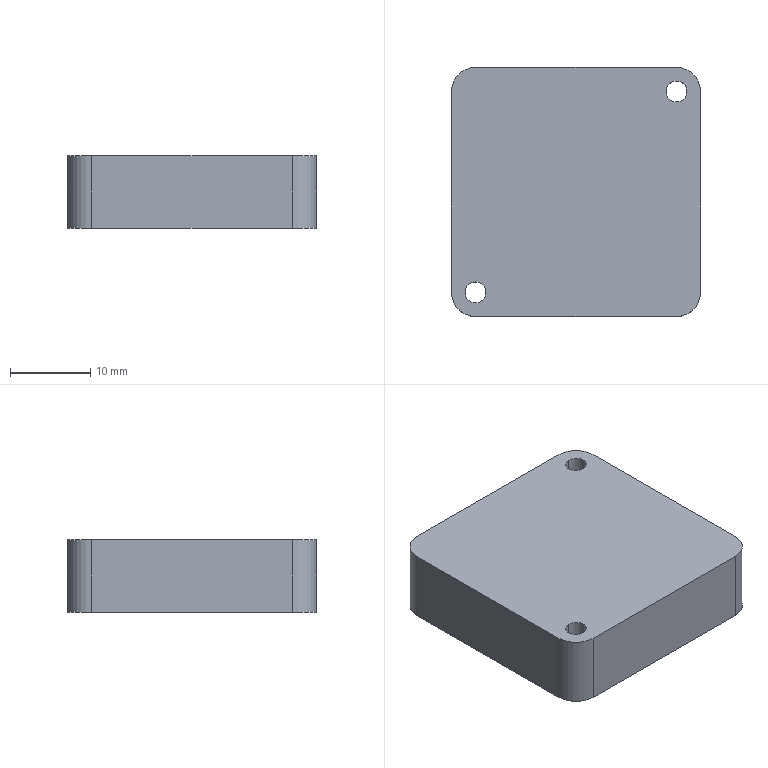Part | NX | 1 solid | 14 faces | box 31 x 31 x 9 mm | volume 8484 mm3 | cylinder 8 | plane 6 | commonest cylinder face diameters 2.6 x4 6 x4
STEP:
#1=CARTESIAN_POINT('',(15.5,12.5,0.));
#2=VERTEX_POINT('',#1);
#3=CARTESIAN_POINT('',(15.5,-12.5,0.));
#4=VERTEX_POINT('',#3);
#5=CARTESIAN_POINT('',(15.5,12.5,0.));
#6=DIRECTION('',(0.,-1.,0.));
#7=VECTOR('',#6,1000.);
#8=LINE('',#5,#7);
#9=EDGE_CURVE('',#2,#4,#8,.T.);
#10=ORIENTED_EDGE('',*,*,#9,.F.);
#11=CARTESIAN_POINT('',(12.5,15.5,0.));
#12=VERTEX_POINT('',#11);
#13=CARTESIAN_POINT('',(12.5,12.5,0.));
#14=DIRECTION('',(0.,0.,1.));
#15=DIRECTION('',(1.,0.,0.));
#16=AXIS2_PLACEMENT_3D('',#13,#14,#15);
#17=CIRCLE('',#16,3.);
#18=EDGE_CURVE('',#2,#12,#17,.T.);
#19=ORIENTED_EDGE('',*,*,#18,.T.);
#20=CARTESIAN_POINT('',(-12.5,15.5,0.));
#21=VERTEX_POINT('',#20);
#22=CARTESIAN_POINT('',(-12.5,15.5,0.));
#23=DIRECTION('',(1.,0.,0.));
#24=VECTOR('',#23,1000.);
#25=LINE('',#22,#24);
#26=EDGE_CURVE('',#21,#12,#25,.T.);
#27=ORIENTED_EDGE('',*,*,#26,.F.);
#28=CARTESIAN_POINT('',(-15.5,12.5,0.));
#29=VERTEX_POINT('',#28);
#30=CARTESIAN_POINT('',(-12.5,12.5,0.));
#31=DIRECTION('',(0.,0.,1.));
#32=DIRECTION('',(0.,1.,0.));
#33=AXIS2_PLACEMENT_3D('',#30,#31,#32);
#34=CIRCLE('',#33,3.);
#35=EDGE_CURVE('',#21,#29,#34,.T.);
#36=ORIENTED_EDGE('',*,*,#35,.T.);
#37=CARTESIAN_POINT('',(-15.5,-12.5,0.));
#38=VERTEX_POINT('',#37);
#39=CARTESIAN_POINT('',(-15.5,-12.5,0.));
#40=DIRECTION('',(0.,1.,0.));
#41=VECTOR('',#40,1000.);
#42=LINE('',#39,#41);
#43=EDGE_CURVE('',#38,#29,#42,.T.);
#44=ORIENTED_EDGE('',*,*,#43,.F.);
#45=CARTESIAN_POINT('',(-12.5,-15.5,0.));
#46=VERTEX_POINT('',#45);
#47=CARTESIAN_POINT('',(-12.5,-12.5,0.));
#48=DIRECTION('',(0.,0.,1.));
#49=DIRECTION('',(-1.,0.,0.));
#50=AXIS2_PLACEMENT_3D('',#47,#48,#49);
#51=CIRCLE('',#50,3.);
#52=EDGE_CURVE('',#38,#46,#51,.T.);
#53=ORIENTED_EDGE('',*,*,#52,.T.);
#54=CARTESIAN_POINT('',(12.5,-15.5,0.));
#55=VERTEX_POINT('',#54);
#56=CARTESIAN_POINT('',(12.5,-15.5,0.));
#57=DIRECTION('',(-1.,0.,0.));
#58=VECTOR('',#57,1000.);
#59=LINE('',#56,#58);
#60=EDGE_CURVE('',#55,#46,#59,.T.);
#61=ORIENTED_EDGE('',*,*,#60,.F.);
#62=CARTESIAN_POINT('',(12.5,-12.5,0.));
#63=DIRECTION('',(0.,0.,1.));
#64=DIRECTION('',(0.,-1.,0.));
#65=AXIS2_PLACEMENT_3D('',#62,#63,#64);
#66=CIRCLE('',#65,3.);
#67=EDGE_CURVE('',#55,#4,#66,.T.);
#68=ORIENTED_EDGE('',*,*,#67,.T.);
#69=EDGE_LOOP('',(#10,#19,#27,#36,#44,#53,#61,#68));
#70=FACE_BOUND('',#69,.T.);
#71=CARTESIAN_POINT('',(-12.5,-11.2,0.));
#72=VERTEX_POINT('',#71);
#73=CARTESIAN_POINT('',(-12.5,-13.8,0.));
#74=VERTEX_POINT('',#73);
#75=CARTESIAN_POINT('',(-12.5,-12.5,0.));
#76=DIRECTION('',(0.,0.,-1.));
#77=DIRECTION('',(0.,1.,0.));
#78=AXIS2_PLACEMENT_3D('',#75,#76,#77);
#79=CIRCLE('',#78,1.3);
#80=EDGE_CURVE('',#72,#74,#79,.T.);
#81=ORIENTED_EDGE('',*,*,#80,.T.);
#82=CARTESIAN_POINT('',(-12.5,-12.5,0.));
#83=DIRECTION('',(0.,0.,-1.));
#84=DIRECTION('',(0.,-1.,0.));
#85=AXIS2_PLACEMENT_3D('',#82,#83,#84);
#86=CIRCLE('',#85,1.3);
#87=EDGE_CURVE('',#74,#72,#86,.T.);
#88=ORIENTED_EDGE('',*,*,#87,.T.);
#89=EDGE_LOOP('',(#81,#88));
#90=FACE_BOUND('',#89,.T.);
#91=CARTESIAN_POINT('',(12.5,13.8,0.));
#92=VERTEX_POINT('',#91);
#93=CARTESIAN_POINT('',(12.5,11.2,0.));
#94=VERTEX_POINT('',#93);
#95=CARTESIAN_POINT('',(12.5,12.5,0.));
#96=DIRECTION('',(0.,0.,-1.));
#97=DIRECTION('',(0.,1.,0.));
#98=AXIS2_PLACEMENT_3D('',#95,#96,#97);
#99=CIRCLE('',#98,1.3);
#100=EDGE_CURVE('',#92,#94,#99,.T.);
#101=ORIENTED_EDGE('',*,*,#100,.T.);
#102=CARTESIAN_POINT('',(12.5,12.5,0.));
#103=DIRECTION('',(0.,0.,-1.));
#104=DIRECTION('',(0.,-1.,0.));
#105=AXIS2_PLACEMENT_3D('',#102,#103,#104);
#106=CIRCLE('',#105,1.3);
#107=EDGE_CURVE('',#94,#92,#106,.T.);
#108=ORIENTED_EDGE('',*,*,#107,.T.);
#109=EDGE_LOOP('',(#101,#108));
#110=FACE_BOUND('',#109,.T.);
#111=CARTESIAN_POINT('',(56.514,13.062,0.));
#112=DIRECTION('',(0.,0.,-1.));
#113=DIRECTION('',(-1.,0.,0.));
#114=AXIS2_PLACEMENT_3D('',#111,#112,#113);
#115=PLANE('',#114);
#116=ADVANCED_FACE('',(#70,#90,#110),#115,.F.);
#117=CARTESIAN_POINT('',(12.5,-15.5,-9.));
#118=VERTEX_POINT('',#117);
#119=CARTESIAN_POINT('',(12.5,-15.5,-9.));
#120=DIRECTION('',(0.,0.,1.));
#121=VECTOR('',#120,1000.);
#122=LINE('',#119,#121);
#123=EDGE_CURVE('',#118,#55,#122,.T.);
#124=ORIENTED_EDGE('',*,*,#123,.F.);
#125=CARTESIAN_POINT('',(15.5,-12.5,-9.));
#126=VERTEX_POINT('',#125);
#127=CARTESIAN_POINT('',(12.5,-12.5,-9.));
#128=DIRECTION('',(0.,0.,-1.));
#129=DIRECTION('',(1.,0.,0.));
#130=AXIS2_PLACEMENT_3D('',#127,#128,#129);
#131=CIRCLE('',#130,3.);
#132=EDGE_CURVE('',#126,#118,#131,.T.);
#133=ORIENTED_EDGE('',*,*,#132,.F.);
#134=CARTESIAN_POINT('',(15.5,-12.5,-9.));
#135=DIRECTION('',(0.,0.,1.));
#136=VECTOR('',#135,1000.);
#137=LINE('',#134,#136);
#138=EDGE_CURVE('',#126,#4,#137,.T.);
#139=ORIENTED_EDGE('',*,*,#138,.T.);
#140=ORIENTED_EDGE('',*,*,#67,.F.);
#141=EDGE_LOOP('',(#124,#133,#139,#140));
#142=FACE_BOUND('',#141,.T.);
#143=CARTESIAN_POINT('',(12.5,-12.5,-57.778));
#144=DIRECTION('',(0.,0.,1.));
#145=DIRECTION('',(0.,1.,0.));
#146=AXIS2_PLACEMENT_3D('',#143,#144,#145);
#147=CYLINDRICAL_SURFACE('',#146,3.);
#148=ADVANCED_FACE('',(#142),#147,.T.);
#149=CARTESIAN_POINT('',(15.5,12.5,-9.));
#150=VERTEX_POINT('',#149);
#151=CARTESIAN_POINT('',(15.5,12.5,-9.));
#152=DIRECTION('',(0.,-1.,0.));
#153=VECTOR('',#152,1000.);
#154=LINE('',#151,#153);
#155=EDGE_CURVE('',#150,#126,#154,.T.);
#156=ORIENTED_EDGE('',*,*,#155,.F.);
#157=CARTESIAN_POINT('',(15.5,12.5,-9.));
#158=DIRECTION('',(0.,0.,1.));
#159=VECTOR('',#158,1000.);
#160=LINE('',#157,#159);
#161=EDGE_CURVE('',#150,#2,#160,.T.);
#162=ORIENTED_EDGE('',*,*,#161,.T.);
#163=ORIENTED_EDGE('',*,*,#9,.T.);
#164=ORIENTED_EDGE('',*,*,#138,.F.);
#165=EDGE_LOOP('',(#156,#162,#163,#164));
#166=FACE_BOUND('',#165,.T.);
#167=CARTESIAN_POINT('',(15.5,15.5,0.));
#168=DIRECTION('',(1.,0.,0.));
#169=DIRECTION('',(0.,1.,0.));
#170=AXIS2_PLACEMENT_3D('',#167,#168,#169);
#171=PLANE('',#170);
#172=ADVANCED_FACE('',(#166),#171,.T.);
#173=ORIENTED_EDGE('',*,*,#161,.F.);
#174=CARTESIAN_POINT('',(12.5,15.5,-9.));
#175=VERTEX_POINT('',#174);
#176=CARTESIAN_POINT('',(12.5,12.5,-9.));
#177=DIRECTION('',(0.,0.,-1.));
#178=DIRECTION('',(0.,1.,0.));
#179=AXIS2_PLACEMENT_3D('',#176,#177,#178);
#180=CIRCLE('',#179,3.);
#181=EDGE_CURVE('',#175,#150,#180,.T.);
#182=ORIENTED_EDGE('',*,*,#181,.F.);
#183=CARTESIAN_POINT('',(12.5,15.5,-9.));
#184=DIRECTION('',(0.,0.,1.));
#185=VECTOR('',#184,1000.);
#186=LINE('',#183,#185);
#187=EDGE_CURVE('',#175,#12,#186,.T.);
#188=ORIENTED_EDGE('',*,*,#187,.T.);
#189=ORIENTED_EDGE('',*,*,#18,.F.);
#190=EDGE_LOOP('',(#173,#182,#188,#189));
#191=FACE_BOUND('',#190,.T.);
#192=CARTESIAN_POINT('',(12.5,12.5,-57.778));
#193=DIRECTION('',(0.,0.,1.));
#194=DIRECTION('',(-1.,0.,0.));
#195=AXIS2_PLACEMENT_3D('',#192,#193,#194);
#196=CYLINDRICAL_SURFACE('',#195,3.);
#197=ADVANCED_FACE('',(#191),#196,.T.);
#198=ORIENTED_EDGE('',*,*,#26,.T.);
#199=ORIENTED_EDGE('',*,*,#187,.F.);
#200=CARTESIAN_POINT('',(-12.5,15.5,-9.));
#201=VERTEX_POINT('',#200);
#202=CARTESIAN_POINT('',(-12.5,15.5,-9.));
#203=DIRECTION('',(1.,0.,0.));
#204=VECTOR('',#203,1000.);
#205=LINE('',#202,#204);
#206=EDGE_CURVE('',#201,#175,#205,.T.);
#207=ORIENTED_EDGE('',*,*,#206,.F.);
#208=CARTESIAN_POINT('',(-12.5,15.5,-9.));
#209=DIRECTION('',(0.,0.,1.));
#210=VECTOR('',#209,1000.);
#211=LINE('',#208,#210);
#212=EDGE_CURVE('',#201,#21,#211,.T.);
#213=ORIENTED_EDGE('',*,*,#212,.T.);
#214=EDGE_LOOP('',(#198,#199,#207,#213));
#215=FACE_BOUND('',#214,.T.);
#216=CARTESIAN_POINT('',(-15.5,15.5,0.));
#217=DIRECTION('',(0.,1.,0.));
#218=DIRECTION('',(-1.,0.,0.));
#219=AXIS2_PLACEMENT_3D('',#216,#217,#218);
#220=PLANE('',#219);
#221=ADVANCED_FACE('',(#215),#220,.T.);
#222=ORIENTED_EDGE('',*,*,#212,.F.);
#223=CARTESIAN_POINT('',(-15.5,12.5,-9.));
#224=VERTEX_POINT('',#223);
#225=CARTESIAN_POINT('',(-12.5,12.5,-9.));
#226=DIRECTION('',(0.,0.,-1.));
#227=DIRECTION('',(-1.,0.,0.));
#228=AXIS2_PLACEMENT_3D('',#225,#226,#227);
#229=CIRCLE('',#228,3.);
#230=EDGE_CURVE('',#224,#201,#229,.T.);
#231=ORIENTED_EDGE('',*,*,#230,.F.);
#232=CARTESIAN_POINT('',(-15.5,12.5,-9.));
#233=DIRECTION('',(0.,0.,1.));
#234=VECTOR('',#233,1000.);
#235=LINE('',#232,#234);
#236=EDGE_CURVE('',#224,#29,#235,.T.);
#237=ORIENTED_EDGE('',*,*,#236,.T.);
#238=ORIENTED_EDGE('',*,*,#35,.F.);
#239=EDGE_LOOP('',(#222,#231,#237,#238));
#240=FACE_BOUND('',#239,.T.);
#241=CARTESIAN_POINT('',(-12.5,12.5,-57.778));
#242=DIRECTION('',(0.,0.,1.));
#243=DIRECTION('',(0.,-1.,0.));
#244=AXIS2_PLACEMENT_3D('',#241,#242,#243);
#245=CYLINDRICAL_SURFACE('',#244,3.);
#246=ADVANCED_FACE('',(#240),#245,.T.);
#247=ORIENTED_EDGE('',*,*,#43,.T.);
#248=ORIENTED_EDGE('',*,*,#236,.F.);
#249=CARTESIAN_POINT('',(-15.5,-12.5,-9.));
#250=VERTEX_POINT('',#249);
#251=CARTESIAN_POINT('',(-15.5,-12.5,-9.));
#252=DIRECTION('',(0.,1.,0.));
#253=VECTOR('',#252,1000.);
#254=LINE('',#251,#253);
#255=EDGE_CURVE('',#250,#224,#254,.T.);
#256=ORIENTED_EDGE('',*,*,#255,.F.);
#257=CARTESIAN_POINT('',(-15.5,-12.5,-9.));
#258=DIRECTION('',(0.,0.,1.));
#259=VECTOR('',#258,1000.);
#260=LINE('',#257,#259);
#261=EDGE_CURVE('',#250,#38,#260,.T.);
#262=ORIENTED_EDGE('',*,*,#261,.T.);
#263=EDGE_LOOP('',(#247,#248,#256,#262));
#264=FACE_BOUND('',#263,.T.);
#265=CARTESIAN_POINT('',(-15.5,-15.5,0.));
#266=DIRECTION('',(-1.,0.,0.));
#267=DIRECTION('',(0.,-1.,0.));
#268=AXIS2_PLACEMENT_3D('',#265,#266,#267);
#269=PLANE('',#268);
#270=ADVANCED_FACE('',(#264),#269,.T.);
#271=ORIENTED_EDGE('',*,*,#261,.F.);
#272=CARTESIAN_POINT('',(-12.5,-15.5,-9.));
#273=VERTEX_POINT('',#272);
#274=CARTESIAN_POINT('',(-12.5,-12.5,-9.));
#275=DIRECTION('',(0.,0.,-1.));
#276=DIRECTION('',(0.,-1.,0.));
#277=AXIS2_PLACEMENT_3D('',#274,#275,#276);
#278=CIRCLE('',#277,3.);
#279=EDGE_CURVE('',#273,#250,#278,.T.);
#280=ORIENTED_EDGE('',*,*,#279,.F.);
#281=CARTESIAN_POINT('',(-12.5,-15.5,-9.));
#282=DIRECTION('',(0.,0.,1.));
#283=VECTOR('',#282,1000.);
#284=LINE('',#281,#283);
#285=EDGE_CURVE('',#273,#46,#284,.T.);
#286=ORIENTED_EDGE('',*,*,#285,.T.);
#287=ORIENTED_EDGE('',*,*,#52,.F.);
#288=EDGE_LOOP('',(#271,#280,#286,#287));
#289=FACE_BOUND('',#288,.T.);
#290=CARTESIAN_POINT('',(-12.5,-12.5,-57.778));
#291=DIRECTION('',(0.,0.,1.));
#292=DIRECTION('',(1.,0.,0.));
#293=AXIS2_PLACEMENT_3D('',#290,#291,#292);
#294=CYLINDRICAL_SURFACE('',#293,3.);
#295=ADVANCED_FACE('',(#289),#294,.T.);
#296=ORIENTED_EDGE('',*,*,#60,.T.);
#297=ORIENTED_EDGE('',*,*,#285,.F.);
#298=CARTESIAN_POINT('',(12.5,-15.5,-9.));
#299=DIRECTION('',(-1.,0.,0.));
#300=VECTOR('',#299,1000.);
#301=LINE('',#298,#300);
#302=EDGE_CURVE('',#118,#273,#301,.T.);
#303=ORIENTED_EDGE('',*,*,#302,.F.);
#304=ORIENTED_EDGE('',*,*,#123,.T.);
#305=EDGE_LOOP('',(#296,#297,#303,#304));
#306=FACE_BOUND('',#305,.T.);
#307=CARTESIAN_POINT('',(15.5,-15.5,0.));
#308=DIRECTION('',(0.,-1.,0.));
#309=DIRECTION('',(1.,0.,0.));
#310=AXIS2_PLACEMENT_3D('',#307,#308,#309);
#311=PLANE('',#310);
#312=ADVANCED_FACE('',(#306),#311,.T.);
#313=ORIENTED_EDGE('',*,*,#302,.T.);
#314=ORIENTED_EDGE('',*,*,#279,.T.);
#315=ORIENTED_EDGE('',*,*,#255,.T.);
#316=ORIENTED_EDGE('',*,*,#230,.T.);
#317=ORIENTED_EDGE('',*,*,#206,.T.);
#318=ORIENTED_EDGE('',*,*,#181,.T.);
#319=ORIENTED_EDGE('',*,*,#155,.T.);
#320=ORIENTED_EDGE('',*,*,#132,.T.);
#321=EDGE_LOOP('',(#313,#314,#315,#316,#317,#318,#319,#320));
#322=FACE_BOUND('',#321,.T.);
#323=CARTESIAN_POINT('',(-12.5,-11.2,-9.));
#324=VERTEX_POINT('',#323);
#325=CARTESIAN_POINT('',(-12.5,-13.8,-9.));
#326=VERTEX_POINT('',#325);
#327=CARTESIAN_POINT('',(-12.5,-12.5,-9.));
#328=DIRECTION('',(0.,0.,-1.));
#329=DIRECTION('',(0.,1.,0.));
#330=AXIS2_PLACEMENT_3D('',#327,#328,#329);
#331=CIRCLE('',#330,1.3);
#332=EDGE_CURVE('',#324,#326,#331,.T.);
#333=ORIENTED_EDGE('',*,*,#332,.F.);
#334=CARTESIAN_POINT('',(-12.5,-12.5,-9.));
#335=DIRECTION('',(0.,0.,-1.));
#336=DIRECTION('',(0.,-1.,0.));
#337=AXIS2_PLACEMENT_3D('',#334,#335,#336);
#338=CIRCLE('',#337,1.3);
#339=EDGE_CURVE('',#326,#324,#338,.T.);
#340=ORIENTED_EDGE('',*,*,#339,.F.);
#341=EDGE_LOOP('',(#333,#340));
#342=FACE_BOUND('',#341,.T.);
#343=CARTESIAN_POINT('',(12.5,13.8,-9.));
#344=VERTEX_POINT('',#343);
#345=CARTESIAN_POINT('',(12.5,11.2,-9.));
#346=VERTEX_POINT('',#345);
#347=CARTESIAN_POINT('',(12.5,12.5,-9.));
#348=DIRECTION('',(0.,0.,-1.));
#349=DIRECTION('',(0.,1.,0.));
#350=AXIS2_PLACEMENT_3D('',#347,#348,#349);
#351=CIRCLE('',#350,1.3);
#352=EDGE_CURVE('',#344,#346,#351,.T.);
#353=ORIENTED_EDGE('',*,*,#352,.F.);
#354=CARTESIAN_POINT('',(12.5,12.5,-9.));
#355=DIRECTION('',(0.,0.,-1.));
#356=DIRECTION('',(0.,-1.,0.));
#357=AXIS2_PLACEMENT_3D('',#354,#355,#356);
#358=CIRCLE('',#357,1.3);
#359=EDGE_CURVE('',#346,#344,#358,.T.);
#360=ORIENTED_EDGE('',*,*,#359,.F.);
#361=EDGE_LOOP('',(#353,#360));
#362=FACE_BOUND('',#361,.T.);
#363=CARTESIAN_POINT('',(56.514,15.662,-9.));
#364=DIRECTION('',(0.,0.,-1.));
#365=DIRECTION('',(1.,0.,0.));
#366=AXIS2_PLACEMENT_3D('',#363,#364,#365);
#367=PLANE('',#366);
#368=ADVANCED_FACE('',(#322,#342,#362),#367,.T.);
#369=CARTESIAN_POINT('',(-12.5,-13.8,-9.));
#370=DIRECTION('',(0.,0.,1.));
#371=VECTOR('',#370,1000.);
#372=LINE('',#369,#371);
#373=EDGE_CURVE('',#326,#74,#372,.T.);
#374=ORIENTED_EDGE('',*,*,#373,.F.);
#375=ORIENTED_EDGE('',*,*,#339,.T.);
#376=CARTESIAN_POINT('',(-12.5,-11.2,-9.));
#377=DIRECTION('',(0.,0.,1.));
#378=VECTOR('',#377,1000.);
#379=LINE('',#376,#378);
#380=EDGE_CURVE('',#324,#72,#379,.T.);
#381=ORIENTED_EDGE('',*,*,#380,.T.);
#382=ORIENTED_EDGE('',*,*,#87,.F.);
#383=EDGE_LOOP('',(#374,#375,#381,#382));
#384=FACE_BOUND('',#383,.T.);
#385=CARTESIAN_POINT('',(-12.5,-12.5,-8.5));
#386=DIRECTION('',(0.,0.,-1.));
#387=DIRECTION('',(0.,1.,0.));
#388=AXIS2_PLACEMENT_3D('',#385,#386,#387);
#389=CYLINDRICAL_SURFACE('',#388,1.3);
#390=ADVANCED_FACE('',(#384),#389,.F.);
#391=ORIENTED_EDGE('',*,*,#380,.F.);
#392=ORIENTED_EDGE('',*,*,#332,.T.);
#393=ORIENTED_EDGE('',*,*,#373,.T.);
#394=ORIENTED_EDGE('',*,*,#80,.F.);
#395=EDGE_LOOP('',(#391,#392,#393,#394));
#396=FACE_BOUND('',#395,.T.);
#397=CARTESIAN_POINT('',(-12.5,-12.5,-8.5));
#398=DIRECTION('',(0.,0.,-1.));
#399=DIRECTION('',(0.,1.,0.));
#400=AXIS2_PLACEMENT_3D('',#397,#398,#399);
#401=CYLINDRICAL_SURFACE('',#400,1.3);
#402=ADVANCED_FACE('',(#396),#401,.F.);
#403=CARTESIAN_POINT('',(12.5,11.2,-9.));
#404=DIRECTION('',(0.,0.,1.));
#405=VECTOR('',#404,1000.);
#406=LINE('',#403,#405);
#407=EDGE_CURVE('',#346,#94,#406,.T.);
#408=ORIENTED_EDGE('',*,*,#407,.F.);
#409=ORIENTED_EDGE('',*,*,#359,.T.);
#410=CARTESIAN_POINT('',(12.5,13.8,-9.));
#411=DIRECTION('',(0.,0.,1.));
#412=VECTOR('',#411,1000.);
#413=LINE('',#410,#412);
#414=EDGE_CURVE('',#344,#92,#413,.T.);
#415=ORIENTED_EDGE('',*,*,#414,.T.);
#416=ORIENTED_EDGE('',*,*,#107,.F.);
#417=EDGE_LOOP('',(#408,#409,#415,#416));
#418=FACE_BOUND('',#417,.T.);
#419=CARTESIAN_POINT('',(12.5,12.5,-8.5));
#420=DIRECTION('',(0.,0.,-1.));
#421=DIRECTION('',(0.,1.,0.));
#422=AXIS2_PLACEMENT_3D('',#419,#420,#421);
#423=CYLINDRICAL_SURFACE('',#422,1.3);
#424=ADVANCED_FACE('',(#418),#423,.F.);
#425=ORIENTED_EDGE('',*,*,#414,.F.);
#426=ORIENTED_EDGE('',*,*,#352,.T.);
#427=ORIENTED_EDGE('',*,*,#407,.T.);
#428=ORIENTED_EDGE('',*,*,#100,.F.);
#429=EDGE_LOOP('',(#425,#426,#427,#428));
#430=FACE_BOUND('',#429,.T.);
#431=CARTESIAN_POINT('',(12.5,12.5,-8.5));
#432=DIRECTION('',(0.,0.,-1.));
#433=DIRECTION('',(0.,1.,0.));
#434=AXIS2_PLACEMENT_3D('',#431,#432,#433);
#435=CYLINDRICAL_SURFACE('',#434,1.3);
#436=ADVANCED_FACE('',(#430),#435,.F.);
#437=CLOSED_SHELL('',(#116,#148,#172,#197,#221,#246,#270,#295,#312,#368,#390,#402,#424,#436));
#438=MANIFOLD_SOLID_BREP('',#437);
#439=(LENGTH_UNIT()NAMED_UNIT(*)SI_UNIT(.MILLI.,.METRE.));
#440=UNCERTAINTY_MEASURE_WITH_UNIT(LENGTH_MEASURE(0.00001),#439,'','');
#441=(NAMED_UNIT(*)PLANE_ANGLE_UNIT()SI_UNIT($,.RADIAN.));
#442=(NAMED_UNIT(*)SI_UNIT($,.STERADIAN.)SOLID_ANGLE_UNIT());
#443=(GEOMETRIC_REPRESENTATION_CONTEXT(3)GLOBAL_UNCERTAINTY_ASSIGNED_CONTEXT((#440))GLOBAL_UNIT_ASSIGNED_CONTEXT((#439,#441,#442))REPRESENTATION_CONTEXT('',''));
#444=ADVANCED_BREP_SHAPE_REPRESENTATION('',(#438),#443);